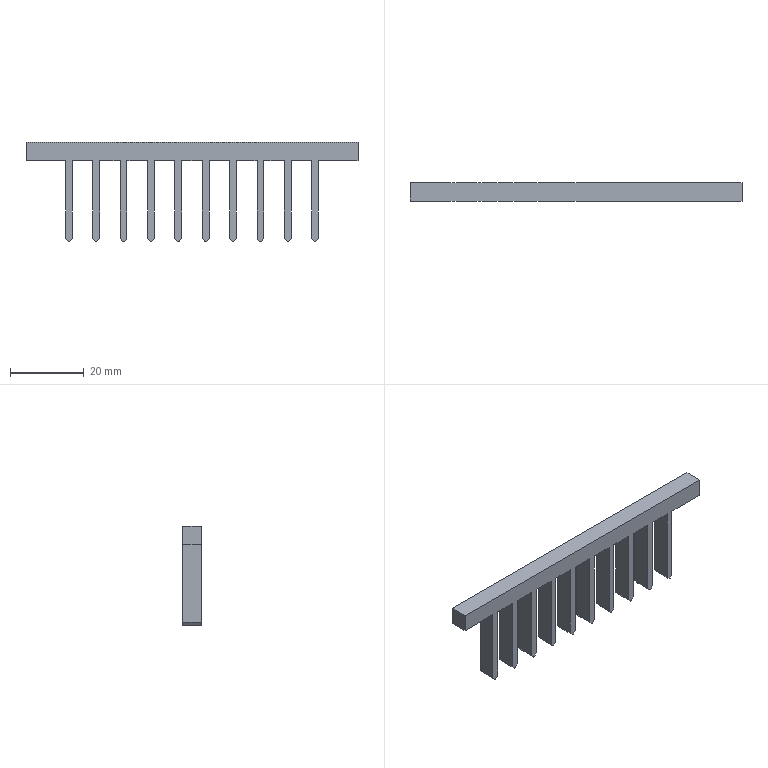Part | STEP file | 200 mesh_id1886 | 1 solid | 66 faces | box 90 x 4.94 x 26.94 mm | volume 4137 mm3 | plane 56 | cylinder 10 | commonest cylinder face diameters 0.5 x10